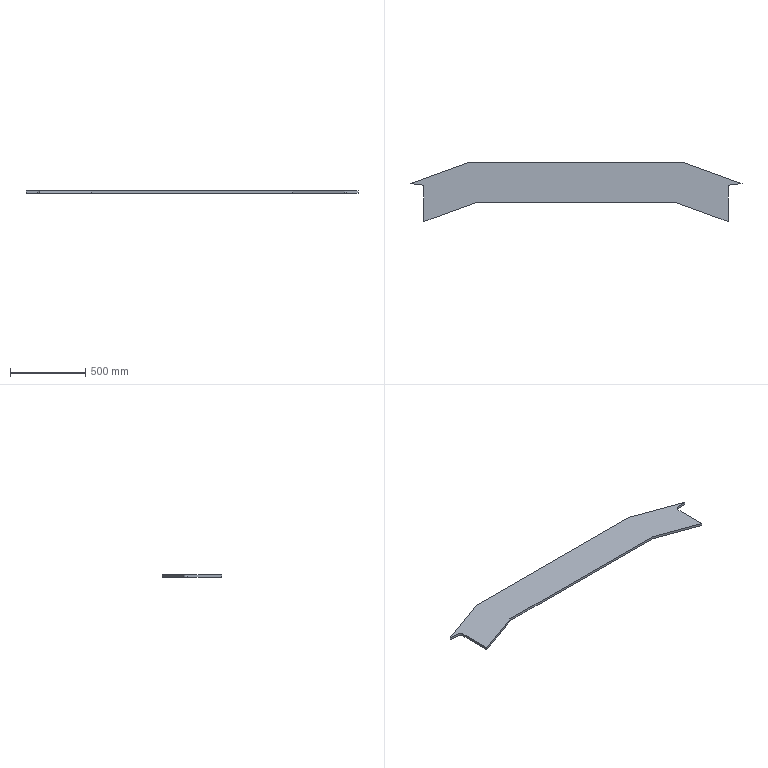Part | SolidWorks | features Fillet 1, FlatPattern 1, ICE 1, SMBaseFlange 1, SheetMetal 1 | 1 solid | 14 faces | box 2205 x 392.571 x 16 mm | volume 8902489 mm3 | plane 12 | cylinder 2 | commonest cylinder face diameters 40 x2
STEP:
#1=CARTESIAN_POINT('',(715.,0.,0.));
#2=VERTEX_POINT('',#1);
#3=CARTESIAN_POINT('',(-715.,0.,0.));
#4=VERTEX_POINT('',#3);
#5=CARTESIAN_POINT('',(-715.,0.,0.));
#6=DIRECTION('',(-1.,0.,0.));
#7=VECTOR('',#6,1000.);
#8=LINE('',#5,#7);
#9=EDGE_CURVE('',#2,#4,#8,.T.);
#10=ORIENTED_EDGE('',*,*,#9,.F.);
#11=CARTESIAN_POINT('',(715.,0.,-16.));
#12=VERTEX_POINT('',#11);
#13=CARTESIAN_POINT('',(715.,0.,-16.));
#14=DIRECTION('',(0.,0.,1.));
#15=VECTOR('',#14,1000.);
#16=LINE('',#13,#15);
#17=EDGE_CURVE('',#12,#2,#16,.T.);
#18=ORIENTED_EDGE('',*,*,#17,.F.);
#19=CARTESIAN_POINT('',(-715.,0.,-16.));
#20=VERTEX_POINT('',#19);
#21=CARTESIAN_POINT('',(-715.,0.,-16.));
#22=DIRECTION('',(-1.,0.,0.));
#23=VECTOR('',#22,1000.);
#24=LINE('',#21,#23);
#25=EDGE_CURVE('',#12,#20,#24,.T.);
#26=ORIENTED_EDGE('',*,*,#25,.T.);
#27=CARTESIAN_POINT('',(-715.,0.,-16.));
#28=DIRECTION('',(0.,0.,1.));
#29=VECTOR('',#28,1000.);
#30=LINE('',#27,#29);
#31=EDGE_CURVE('',#20,#4,#30,.T.);
#32=ORIENTED_EDGE('',*,*,#31,.T.);
#33=EDGE_LOOP('',(#10,#18,#26,#32));
#34=FACE_OUTER_BOUND('',#33,.T.);
#35=CARTESIAN_POINT('',(-715.,0.,-16.));
#36=DIRECTION('',(0.,1.,0.));
#37=DIRECTION('',(0.,0.,1.));
#38=AXIS2_PLACEMENT_3D('',#35,#36,#37);
#39=PLANE('',#38);
#40=ADVANCED_FACE('',(#34),#39,.T.);
#41=CARTESIAN_POINT('',(1102.619,-141.082,-16.));
#42=VERTEX_POINT('',#41);
#43=CARTESIAN_POINT('',(1102.619,-141.082,0.));
#44=VERTEX_POINT('',#43);
#45=CARTESIAN_POINT('',(1102.619,-141.082,-16.));
#46=DIRECTION('',(0.,0.,1.));
#47=VECTOR('',#46,1000.);
#48=LINE('',#45,#47);
#49=EDGE_CURVE('',#42,#44,#48,.T.);
#50=ORIENTED_EDGE('',*,*,#49,.F.);
#51=CARTESIAN_POINT('',(715.,0.,-16.));
#52=DIRECTION('',(-0.9397,0.342,0.));
#53=VECTOR('',#52,1000.);
#54=LINE('',#51,#53);
#55=EDGE_CURVE('',#42,#12,#54,.T.);
#56=ORIENTED_EDGE('',*,*,#55,.T.);
#57=ORIENTED_EDGE('',*,*,#17,.T.);
#58=CARTESIAN_POINT('',(715.,0.,0.));
#59=DIRECTION('',(-0.9397,0.342,0.));
#60=VECTOR('',#59,1000.);
#61=LINE('',#58,#60);
#62=EDGE_CURVE('',#44,#2,#61,.T.);
#63=ORIENTED_EDGE('',*,*,#62,.F.);
#64=EDGE_LOOP('',(#50,#56,#57,#63));
#65=FACE_OUTER_BOUND('',#64,.T.);
#66=CARTESIAN_POINT('',(715.,0.,-16.));
#67=DIRECTION('',(0.342,0.9397,0.));
#68=DIRECTION('',(-0.9397,0.342,0.));
#69=AXIS2_PLACEMENT_3D('',#66,#67,#68);
#70=PLANE('',#69);
#71=ADVANCED_FACE('',(#65),#70,.T.);
#72=CARTESIAN_POINT('',(1010.,-392.571,0.));
#73=VERTEX_POINT('',#72);
#74=CARTESIAN_POINT('',(1010.,-392.571,-16.));
#75=VERTEX_POINT('',#74);
#76=CARTESIAN_POINT('',(1010.,-392.571,-16.));
#77=DIRECTION('',(0.,0.,-1.));
#78=VECTOR('',#77,1000.);
#79=LINE('',#76,#78);
#80=EDGE_CURVE('',#73,#75,#79,.T.);
#81=ORIENTED_EDGE('',*,*,#80,.F.);
#82=CARTESIAN_POINT('',(667.744,-268.,0.));
#83=VERTEX_POINT('',#82);
#84=CARTESIAN_POINT('',(667.744,-268.,0.));
#85=DIRECTION('',(0.9397,-0.342,0.));
#86=VECTOR('',#85,1000.);
#87=LINE('',#84,#86);
#88=EDGE_CURVE('',#83,#73,#87,.T.);
#89=ORIENTED_EDGE('',*,*,#88,.F.);
#90=CARTESIAN_POINT('',(667.744,-268.,-16.));
#91=VERTEX_POINT('',#90);
#92=CARTESIAN_POINT('',(667.744,-268.,-16.));
#93=DIRECTION('',(0.,0.,1.));
#94=VECTOR('',#93,1000.);
#95=LINE('',#92,#94);
#96=EDGE_CURVE('',#91,#83,#95,.T.);
#97=ORIENTED_EDGE('',*,*,#96,.F.);
#98=CARTESIAN_POINT('',(667.744,-268.,-16.));
#99=DIRECTION('',(0.9397,-0.342,0.));
#100=VECTOR('',#99,1000.);
#101=LINE('',#98,#100);
#102=EDGE_CURVE('',#91,#75,#101,.T.);
#103=ORIENTED_EDGE('',*,*,#102,.T.);
#104=EDGE_LOOP('',(#81,#89,#97,#103));
#105=FACE_OUTER_BOUND('',#104,.T.);
#106=CARTESIAN_POINT('',(667.744,-268.,-16.));
#107=DIRECTION('',(-0.342,-0.9397,0.));
#108=DIRECTION('',(0.9397,-0.342,0.));
#109=AXIS2_PLACEMENT_3D('',#106,#107,#108);
#110=PLANE('',#109);
#111=ADVANCED_FACE('',(#105),#110,.T.);
#112=CARTESIAN_POINT('',(-667.744,-268.,0.));
#113=VERTEX_POINT('',#112);
#114=CARTESIAN_POINT('',(-667.744,-268.,0.));
#115=DIRECTION('',(1.,0.,0.));
#116=VECTOR('',#115,1000.);
#117=LINE('',#114,#116);
#118=EDGE_CURVE('',#113,#83,#117,.T.);
#119=ORIENTED_EDGE('',*,*,#118,.F.);
#120=CARTESIAN_POINT('',(-667.744,-268.,-16.));
#121=VERTEX_POINT('',#120);
#122=CARTESIAN_POINT('',(-667.744,-268.,-16.));
#123=DIRECTION('',(0.,0.,1.));
#124=VECTOR('',#123,1000.);
#125=LINE('',#122,#124);
#126=EDGE_CURVE('',#121,#113,#125,.T.);
#127=ORIENTED_EDGE('',*,*,#126,.F.);
#128=CARTESIAN_POINT('',(-667.744,-268.,-16.));
#129=DIRECTION('',(1.,0.,0.));
#130=VECTOR('',#129,1000.);
#131=LINE('',#128,#130);
#132=EDGE_CURVE('',#121,#91,#131,.T.);
#133=ORIENTED_EDGE('',*,*,#132,.T.);
#134=ORIENTED_EDGE('',*,*,#96,.T.);
#135=EDGE_LOOP('',(#119,#127,#133,#134));
#136=FACE_OUTER_BOUND('',#135,.T.);
#137=CARTESIAN_POINT('',(-667.744,-268.,-16.));
#138=DIRECTION('',(0.,-1.,0.));
#139=DIRECTION('',(0.,0.,-1.));
#140=AXIS2_PLACEMENT_3D('',#137,#138,#139);
#141=PLANE('',#140);
#142=ADVANCED_FACE('',(#136),#141,.T.);
#143=CARTESIAN_POINT('',(-1010.,-392.571,-16.));
#144=VERTEX_POINT('',#143);
#145=CARTESIAN_POINT('',(-1010.,-392.571,0.));
#146=VERTEX_POINT('',#145);
#147=CARTESIAN_POINT('',(-1010.,-392.571,-16.));
#148=DIRECTION('',(0.,0.,1.));
#149=VECTOR('',#148,1000.);
#150=LINE('',#147,#149);
#151=EDGE_CURVE('',#144,#146,#150,.T.);
#152=ORIENTED_EDGE('',*,*,#151,.F.);
#153=CARTESIAN_POINT('',(-667.744,-268.,-16.));
#154=DIRECTION('',(0.9397,0.342,0.));
#155=VECTOR('',#154,1000.);
#156=LINE('',#153,#155);
#157=EDGE_CURVE('',#144,#121,#156,.T.);
#158=ORIENTED_EDGE('',*,*,#157,.T.);
#159=ORIENTED_EDGE('',*,*,#126,.T.);
#160=CARTESIAN_POINT('',(-667.744,-268.,0.));
#161=DIRECTION('',(0.9397,0.342,0.));
#162=VECTOR('',#161,1000.);
#163=LINE('',#160,#162);
#164=EDGE_CURVE('',#146,#113,#163,.T.);
#165=ORIENTED_EDGE('',*,*,#164,.F.);
#166=EDGE_LOOP('',(#152,#158,#159,#165));
#167=FACE_OUTER_BOUND('',#166,.T.);
#168=CARTESIAN_POINT('',(-667.744,-268.,-16.));
#169=DIRECTION('',(0.342,-0.9397,0.));
#170=DIRECTION('',(0.9397,0.342,0.));
#171=AXIS2_PLACEMENT_3D('',#168,#169,#170);
#172=PLANE('',#171);
#173=ADVANCED_FACE('',(#167),#172,.T.);
#174=CARTESIAN_POINT('',(-1102.619,-141.082,0.));
#175=VERTEX_POINT('',#174);
#176=CARTESIAN_POINT('',(-1102.619,-141.082,-16.));
#177=VERTEX_POINT('',#176);
#178=CARTESIAN_POINT('',(-1102.619,-141.082,-16.));
#179=DIRECTION('',(0.,0.,-1.));
#180=VECTOR('',#179,1000.);
#181=LINE('',#178,#180);
#182=EDGE_CURVE('',#175,#177,#181,.T.);
#183=ORIENTED_EDGE('',*,*,#182,.F.);
#184=CARTESIAN_POINT('',(-715.,0.,0.));
#185=DIRECTION('',(-0.9397,-0.342,0.));
#186=VECTOR('',#185,1000.);
#187=LINE('',#184,#186);
#188=EDGE_CURVE('',#4,#175,#187,.T.);
#189=ORIENTED_EDGE('',*,*,#188,.F.);
#190=ORIENTED_EDGE('',*,*,#31,.F.);
#191=CARTESIAN_POINT('',(-715.,0.,-16.));
#192=DIRECTION('',(-0.9397,-0.342,0.));
#193=VECTOR('',#192,1000.);
#194=LINE('',#191,#193);
#195=EDGE_CURVE('',#20,#177,#194,.T.);
#196=ORIENTED_EDGE('',*,*,#195,.T.);
#197=EDGE_LOOP('',(#183,#189,#190,#196));
#198=FACE_OUTER_BOUND('',#197,.T.);
#199=CARTESIAN_POINT('',(-715.,0.,-16.));
#200=DIRECTION('',(-0.342,0.9397,0.));
#201=DIRECTION('',(-0.9397,-0.342,0.));
#202=AXIS2_PLACEMENT_3D('',#199,#200,#201);
#203=PLANE('',#202);
#204=ADVANCED_FACE('',(#198),#203,.T.);
#205=CARTESIAN_POINT('',(-1010.,-168.167,-16.));
#206=VERTEX_POINT('',#205);
#207=CARTESIAN_POINT('',(-1010.,-150.,-16.));
#208=DIRECTION('',(0.,1.,0.));
#209=VECTOR('',#208,1000.);
#210=LINE('',#207,#209);
#211=EDGE_CURVE('',#144,#206,#210,.T.);
#212=ORIENTED_EDGE('',*,*,#211,.T.);
#213=CARTESIAN_POINT('',(-1028.083,-148.259,-16.));
#214=VERTEX_POINT('',#213);
#215=CARTESIAN_POINT('',(-1030.,-168.167,-16.));
#216=DIRECTION('',(0.,0.,1.));
#217=DIRECTION('',(1.,0.,0.));
#218=AXIS2_PLACEMENT_3D('',#215,#216,#217);
#219=CIRCLE('',#218,20.);
#220=EDGE_CURVE('',#206,#214,#219,.T.);
#221=ORIENTED_EDGE('',*,*,#220,.T.);
#222=CARTESIAN_POINT('',(-1310.,-121.113,-16.));
#223=DIRECTION('',(-0.9954,0.09585,0.));
#224=VECTOR('',#223,1000.);
#225=LINE('',#222,#224);
#226=EDGE_CURVE('',#214,#177,#225,.T.);
#227=ORIENTED_EDGE('',*,*,#226,.T.);
#228=ORIENTED_EDGE('',*,*,#195,.F.);
#229=ORIENTED_EDGE('',*,*,#25,.F.);
#230=ORIENTED_EDGE('',*,*,#55,.F.);
#231=CARTESIAN_POINT('',(1028.083,-148.259,-16.));
#232=VERTEX_POINT('',#231);
#233=CARTESIAN_POINT('',(1310.,-121.113,-16.));
#234=DIRECTION('',(-0.9954,-0.09585,0.));
#235=VECTOR('',#234,1000.);
#236=LINE('',#233,#235);
#237=EDGE_CURVE('',#42,#232,#236,.T.);
#238=ORIENTED_EDGE('',*,*,#237,.T.);
#239=CARTESIAN_POINT('',(1010.,-168.167,-16.));
#240=VERTEX_POINT('',#239);
#241=CARTESIAN_POINT('',(1030.,-168.167,-16.));
#242=DIRECTION('',(0.,0.,1.));
#243=DIRECTION('',(1.,0.,0.));
#244=AXIS2_PLACEMENT_3D('',#241,#242,#243);
#245=CIRCLE('',#244,20.);
#246=EDGE_CURVE('',#232,#240,#245,.T.);
#247=ORIENTED_EDGE('',*,*,#246,.T.);
#248=CARTESIAN_POINT('',(1010.,-150.,-16.));
#249=DIRECTION('',(0.,-1.,0.));
#250=VECTOR('',#249,1000.);
#251=LINE('',#248,#250);
#252=EDGE_CURVE('',#240,#75,#251,.T.);
#253=ORIENTED_EDGE('',*,*,#252,.T.);
#254=ORIENTED_EDGE('',*,*,#102,.F.);
#255=ORIENTED_EDGE('',*,*,#132,.F.);
#256=ORIENTED_EDGE('',*,*,#157,.F.);
#257=EDGE_LOOP('',(#212,#221,#227,#228,#229,#230,#238,#247,#253,#254,#255,#256));
#258=FACE_OUTER_BOUND('',#257,.T.);
#259=CARTESIAN_POINT('',(0.,0.,-16.));
#260=DIRECTION('',(0.,0.,1.));
#261=DIRECTION('',(1.,0.,0.));
#262=AXIS2_PLACEMENT_3D('',#259,#260,#261);
#263=PLANE('',#262);
#264=ADVANCED_FACE('',(#258),#263,.F.);
#265=CARTESIAN_POINT('',(-1028.083,-148.259,0.));
#266=VERTEX_POINT('',#265);
#267=CARTESIAN_POINT('',(-1310.,-121.113,0.));
#268=DIRECTION('',(-0.9954,0.09585,0.));
#269=VECTOR('',#268,1000.);
#270=LINE('',#267,#269);
#271=EDGE_CURVE('',#266,#175,#270,.T.);
#272=ORIENTED_EDGE('',*,*,#271,.F.);
#273=CARTESIAN_POINT('',(-1010.,-168.167,0.));
#274=VERTEX_POINT('',#273);
#275=CARTESIAN_POINT('',(-1030.,-168.167,0.));
#276=DIRECTION('',(0.,0.,-1.));
#277=DIRECTION('',(1.,0.,0.));
#278=AXIS2_PLACEMENT_3D('',#275,#276,#277);
#279=CIRCLE('',#278,20.);
#280=EDGE_CURVE('',#266,#274,#279,.T.);
#281=ORIENTED_EDGE('',*,*,#280,.T.);
#282=CARTESIAN_POINT('',(-1010.,0.,0.));
#283=DIRECTION('',(0.,1.,0.));
#284=VECTOR('',#283,1000.);
#285=LINE('',#282,#284);
#286=EDGE_CURVE('',#146,#274,#285,.T.);
#287=ORIENTED_EDGE('',*,*,#286,.F.);
#288=ORIENTED_EDGE('',*,*,#164,.T.);
#289=ORIENTED_EDGE('',*,*,#118,.T.);
#290=ORIENTED_EDGE('',*,*,#88,.T.);
#291=CARTESIAN_POINT('',(1010.,-168.167,0.));
#292=VERTEX_POINT('',#291);
#293=CARTESIAN_POINT('',(1010.,-150.,0.));
#294=DIRECTION('',(0.,-1.,0.));
#295=VECTOR('',#294,1000.);
#296=LINE('',#293,#295);
#297=EDGE_CURVE('',#292,#73,#296,.T.);
#298=ORIENTED_EDGE('',*,*,#297,.F.);
#299=CARTESIAN_POINT('',(1028.083,-148.259,0.));
#300=VERTEX_POINT('',#299);
#301=CARTESIAN_POINT('',(1030.,-168.167,0.));
#302=DIRECTION('',(0.,0.,-1.));
#303=DIRECTION('',(1.,0.,0.));
#304=AXIS2_PLACEMENT_3D('',#301,#302,#303);
#305=CIRCLE('',#304,20.);
#306=EDGE_CURVE('',#292,#300,#305,.T.);
#307=ORIENTED_EDGE('',*,*,#306,.T.);
#308=CARTESIAN_POINT('',(23.589,-244.981,0.));
#309=DIRECTION('',(-0.9954,-0.09585,0.));
#310=VECTOR('',#309,1000.);
#311=LINE('',#308,#310);
#312=EDGE_CURVE('',#44,#300,#311,.T.);
#313=ORIENTED_EDGE('',*,*,#312,.F.);
#314=ORIENTED_EDGE('',*,*,#62,.T.);
#315=ORIENTED_EDGE('',*,*,#9,.T.);
#316=ORIENTED_EDGE('',*,*,#188,.T.);
#317=EDGE_LOOP('',(#272,#281,#287,#288,#289,#290,#298,#307,#313,#314,#315,#316));
#318=FACE_OUTER_BOUND('',#317,.T.);
#319=CARTESIAN_POINT('',(0.,0.,0.));
#320=DIRECTION('',(0.,0.,1.));
#321=DIRECTION('',(1.,0.,0.));
#322=AXIS2_PLACEMENT_3D('',#319,#320,#321);
#323=PLANE('',#322);
#324=ADVANCED_FACE('',(#318),#323,.T.);
#325=ORIENTED_EDGE('',*,*,#252,.F.);
#326=CARTESIAN_POINT('',(1010.,-168.167,0.));
#327=DIRECTION('',(0.,0.,1.));
#328=VECTOR('',#327,1000.);
#329=LINE('',#326,#328);
#330=EDGE_CURVE('',#240,#292,#329,.T.);
#331=ORIENTED_EDGE('',*,*,#330,.T.);
#332=ORIENTED_EDGE('',*,*,#297,.T.);
#333=ORIENTED_EDGE('',*,*,#80,.T.);
#334=EDGE_LOOP('',(#325,#331,#332,#333));
#335=FACE_OUTER_BOUND('',#334,.T.);
#336=CARTESIAN_POINT('',(1010.,-150.,-16.));
#337=DIRECTION('',(-1.,0.,0.));
#338=DIRECTION('',(0.,0.,1.));
#339=AXIS2_PLACEMENT_3D('',#336,#337,#338);
#340=PLANE('',#339);
#341=ADVANCED_FACE('',(#335),#340,.F.);
#342=ORIENTED_EDGE('',*,*,#312,.T.);
#343=CARTESIAN_POINT('',(1028.083,-148.259,-16.));
#344=DIRECTION('',(0.,0.,-1.));
#345=VECTOR('',#344,1000.);
#346=LINE('',#343,#345);
#347=EDGE_CURVE('',#300,#232,#346,.T.);
#348=ORIENTED_EDGE('',*,*,#347,.T.);
#349=ORIENTED_EDGE('',*,*,#237,.F.);
#350=ORIENTED_EDGE('',*,*,#49,.T.);
#351=EDGE_LOOP('',(#342,#348,#349,#350));
#352=FACE_OUTER_BOUND('',#351,.T.);
#353=CARTESIAN_POINT('',(1310.,-121.113,-16.));
#354=DIRECTION('',(-0.09585,0.9954,0.));
#355=DIRECTION('',(-0.9954,-0.09585,0.));
#356=AXIS2_PLACEMENT_3D('',#353,#354,#355);
#357=PLANE('',#356);
#358=ADVANCED_FACE('',(#352),#357,.F.);
#359=ORIENTED_EDGE('',*,*,#226,.F.);
#360=CARTESIAN_POINT('',(-1028.083,-148.259,0.));
#361=DIRECTION('',(0.,0.,1.));
#362=VECTOR('',#361,1000.);
#363=LINE('',#360,#362);
#364=EDGE_CURVE('',#214,#266,#363,.T.);
#365=ORIENTED_EDGE('',*,*,#364,.T.);
#366=ORIENTED_EDGE('',*,*,#271,.T.);
#367=ORIENTED_EDGE('',*,*,#182,.T.);
#368=EDGE_LOOP('',(#359,#365,#366,#367));
#369=FACE_OUTER_BOUND('',#368,.T.);
#370=CARTESIAN_POINT('',(-1310.,-121.113,-16.));
#371=DIRECTION('',(0.09585,0.9954,0.));
#372=DIRECTION('',(-0.9954,0.09585,0.));
#373=AXIS2_PLACEMENT_3D('',#370,#371,#372);
#374=PLANE('',#373);
#375=ADVANCED_FACE('',(#369),#374,.F.);
#376=ORIENTED_EDGE('',*,*,#286,.T.);
#377=CARTESIAN_POINT('',(-1010.,-168.167,-16.));
#378=DIRECTION('',(0.,0.,-1.));
#379=VECTOR('',#378,1000.);
#380=LINE('',#377,#379);
#381=EDGE_CURVE('',#274,#206,#380,.T.);
#382=ORIENTED_EDGE('',*,*,#381,.T.);
#383=ORIENTED_EDGE('',*,*,#211,.F.);
#384=ORIENTED_EDGE('',*,*,#151,.T.);
#385=EDGE_LOOP('',(#376,#382,#383,#384));
#386=FACE_OUTER_BOUND('',#385,.T.);
#387=CARTESIAN_POINT('',(-1010.,-150.,-16.));
#388=DIRECTION('',(1.,0.,0.));
#389=DIRECTION('',(0.,1.,0.));
#390=AXIS2_PLACEMENT_3D('',#387,#388,#389);
#391=PLANE('',#390);
#392=ADVANCED_FACE('',(#386),#391,.F.);
#393=ORIENTED_EDGE('',*,*,#246,.F.);
#394=ORIENTED_EDGE('',*,*,#347,.F.);
#395=ORIENTED_EDGE('',*,*,#306,.F.);
#396=ORIENTED_EDGE('',*,*,#330,.F.);
#397=EDGE_LOOP('',(#393,#394,#395,#396));
#398=FACE_OUTER_BOUND('',#397,.T.);
#399=CARTESIAN_POINT('',(1030.,-168.167,-16.));
#400=DIRECTION('',(0.,0.,-1.));
#401=DIRECTION('',(-1.,0.,0.));
#402=AXIS2_PLACEMENT_3D('',#399,#400,#401);
#403=CYLINDRICAL_SURFACE('',#402,20.);
#404=ADVANCED_FACE('',(#398),#403,.F.);
#405=ORIENTED_EDGE('',*,*,#220,.F.);
#406=ORIENTED_EDGE('',*,*,#381,.F.);
#407=ORIENTED_EDGE('',*,*,#280,.F.);
#408=ORIENTED_EDGE('',*,*,#364,.F.);
#409=EDGE_LOOP('',(#405,#406,#407,#408));
#410=FACE_OUTER_BOUND('',#409,.T.);
#411=CARTESIAN_POINT('',(-1030.,-168.167,-16.));
#412=DIRECTION('',(0.,0.,-1.));
#413=DIRECTION('',(-1.,0.,0.));
#414=AXIS2_PLACEMENT_3D('',#411,#412,#413);
#415=CYLINDRICAL_SURFACE('',#414,20.);
#416=ADVANCED_FACE('',(#410),#415,.F.);
#417=CLOSED_SHELL('',(#40,#71,#111,#142,#173,#204,#264,#324,#341,#358,#375,#392,#404,#416));
#418=MANIFOLD_SOLID_BREP('',#417);
#419=CARTESIAN_POINT('',(0.,0.,0.));
#420=DIRECTION('',(0.,0.,1.));
#421=DIRECTION('',(1.,0.,0.));
#422=AXIS2_PLACEMENT_3D('',#419,#420,#421);
#423=(LENGTH_UNIT()NAMED_UNIT(*)SI_UNIT(.MILLI.,.METRE.));
#424=UNCERTAINTY_MEASURE_WITH_UNIT(LENGTH_MEASURE(0.00001),#423,'','');
#425=(NAMED_UNIT(*)PLANE_ANGLE_UNIT()SI_UNIT($,.RADIAN.));
#426=(NAMED_UNIT(*)SI_UNIT($,.STERADIAN.)SOLID_ANGLE_UNIT());
#427=(GEOMETRIC_REPRESENTATION_CONTEXT(3)GLOBAL_UNCERTAINTY_ASSIGNED_CONTEXT((#424))GLOBAL_UNIT_ASSIGNED_CONTEXT((#423,#425,#426))REPRESENTATION_CONTEXT('',''));
#428=ADVANCED_BREP_SHAPE_REPRESENTATION('',(#418,#422),#427);